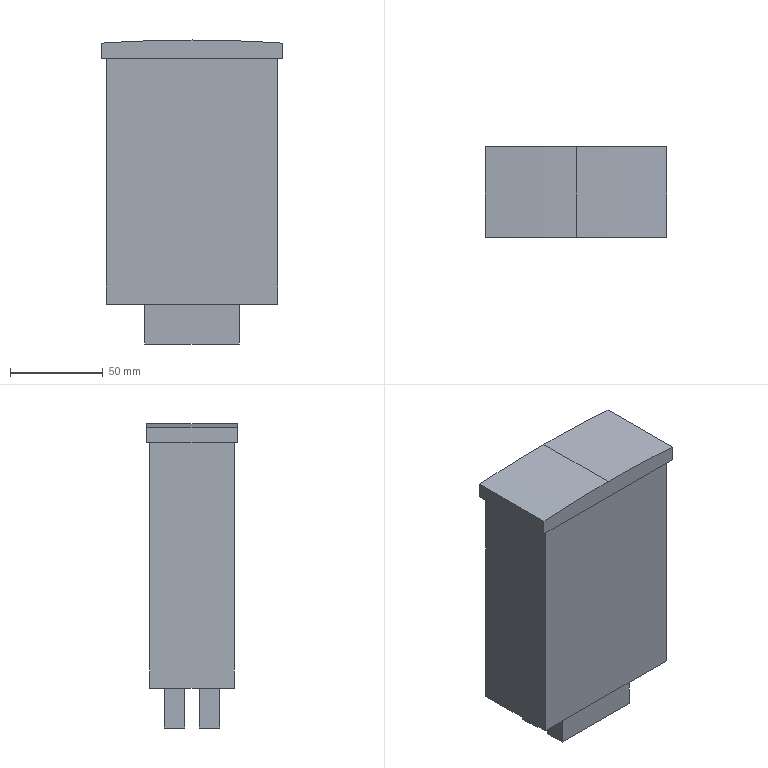Part | SolidWorks | features BaseBody 1 | 1 solid | 22 faces | box 97.6 x 48.9 x 163.5 mm | volume 620484 mm3 | plane 20 | cylinder 2 | commonest cylinder face diameters 1403 x2
STEP:
#1=CARTESIAN_POINT('',(0.,-24.45,71.));
#2=VERTEX_POINT('',#1);
#3=CARTESIAN_POINT('',(-48.8,-24.45,69.3));
#4=VERTEX_POINT('',#3);
#5=CARTESIAN_POINT('',(0.,-24.45,-630.274));
#6=DIRECTION('',(0.,-1.,0.));
#7=DIRECTION('',(0.,0.,1.));
#8=AXIS2_PLACEMENT_3D('',#5,#6,#7);
#9=CIRCLE('',#8,701.274);
#10=EDGE_CURVE('',#2,#4,#9,.T.);
#11=ORIENTED_EDGE('',*,*,#10,.F.);
#12=CARTESIAN_POINT('',(0.,24.45,71.));
#13=VERTEX_POINT('',#12);
#14=CARTESIAN_POINT('',(0.,-24.45,71.));
#15=DIRECTION('',(0.,1.,0.));
#16=VECTOR('',#15,1000.);
#17=LINE('',#14,#16);
#18=EDGE_CURVE('',#2,#13,#17,.T.);
#19=ORIENTED_EDGE('',*,*,#18,.T.);
#20=CARTESIAN_POINT('',(-48.8,24.45,69.3));
#21=VERTEX_POINT('',#20);
#22=CARTESIAN_POINT('',(0.,24.45,-630.274));
#23=DIRECTION('',(0.,-1.,0.));
#24=DIRECTION('',(0.,0.,1.));
#25=AXIS2_PLACEMENT_3D('',#22,#23,#24);
#26=CIRCLE('',#25,701.274);
#27=EDGE_CURVE('',#13,#21,#26,.T.);
#28=ORIENTED_EDGE('',*,*,#27,.T.);
#29=CARTESIAN_POINT('',(-48.8,-24.45,69.3));
#30=DIRECTION('',(0.,1.,0.));
#31=VECTOR('',#30,1000.);
#32=LINE('',#29,#31);
#33=EDGE_CURVE('',#4,#21,#32,.T.);
#34=ORIENTED_EDGE('',*,*,#33,.F.);
#35=EDGE_LOOP('',(#11,#19,#28,#34));
#36=FACE_OUTER_BOUND('',#35,.T.);
#37=CARTESIAN_POINT('',(0.,-24.45,-630.274));
#38=DIRECTION('',(0.,1.,0.));
#39=DIRECTION('',(0.,0.,1.));
#40=AXIS2_PLACEMENT_3D('',#37,#38,#39);
#41=CYLINDRICAL_SURFACE('',#40,701.274);
#42=ADVANCED_FACE('',(#36),#41,.T.);
#43=CARTESIAN_POINT('',(-25.5,-15.,-92.5));
#44=VERTEX_POINT('',#43);
#45=CARTESIAN_POINT('',(-25.5,-4.,-92.5));
#46=VERTEX_POINT('',#45);
#47=CARTESIAN_POINT('',(-25.5,-15.,-92.5));
#48=DIRECTION('',(0.,1.,0.));
#49=VECTOR('',#48,1000.);
#50=LINE('',#47,#49);
#51=EDGE_CURVE('',#44,#46,#50,.T.);
#52=ORIENTED_EDGE('',*,*,#51,.T.);
#53=CARTESIAN_POINT('',(25.5,-4.,-92.5));
#54=VERTEX_POINT('',#53);
#55=CARTESIAN_POINT('',(25.5,-4.,-92.5));
#56=DIRECTION('',(1.,0.,0.));
#57=VECTOR('',#56,1000.);
#58=LINE('',#55,#57);
#59=EDGE_CURVE('',#46,#54,#58,.T.);
#60=ORIENTED_EDGE('',*,*,#59,.T.);
#61=CARTESIAN_POINT('',(25.5,-15.,-92.5));
#62=VERTEX_POINT('',#61);
#63=CARTESIAN_POINT('',(25.5,-15.,-92.5));
#64=DIRECTION('',(0.,-1.,0.));
#65=VECTOR('',#64,1000.);
#66=LINE('',#63,#65);
#67=EDGE_CURVE('',#54,#62,#66,.T.);
#68=ORIENTED_EDGE('',*,*,#67,.T.);
#69=CARTESIAN_POINT('',(25.5,-15.,-92.5));
#70=DIRECTION('',(-1.,0.,0.));
#71=VECTOR('',#70,1000.);
#72=LINE('',#69,#71);
#73=EDGE_CURVE('',#62,#44,#72,.T.);
#74=ORIENTED_EDGE('',*,*,#73,.T.);
#75=EDGE_LOOP('',(#52,#60,#68,#74));
#76=FACE_OUTER_BOUND('',#75,.T.);
#77=CARTESIAN_POINT('',(0.,0.,-92.5));
#78=DIRECTION('',(0.,0.,1.));
#79=DIRECTION('',(1.,0.,0.));
#80=AXIS2_PLACEMENT_3D('',#77,#78,#79);
#81=PLANE('',#80);
#82=ADVANCED_FACE('',(#76),#81,.F.);
#83=CARTESIAN_POINT('',(25.5,-15.,-71.));
#84=VERTEX_POINT('',#83);
#85=CARTESIAN_POINT('',(-25.5,-15.,-71.));
#86=VERTEX_POINT('',#85);
#87=CARTESIAN_POINT('',(25.5,-15.,-71.));
#88=DIRECTION('',(-1.,0.,0.));
#89=VECTOR('',#88,1000.);
#90=LINE('',#87,#89);
#91=EDGE_CURVE('',#84,#86,#90,.T.);
#92=ORIENTED_EDGE('',*,*,#91,.T.);
#93=CARTESIAN_POINT('',(-25.5,-15.,-92.5));
#94=DIRECTION('',(0.,0.,1.));
#95=VECTOR('',#94,1000.);
#96=LINE('',#93,#95);
#97=EDGE_CURVE('',#44,#86,#96,.T.);
#98=ORIENTED_EDGE('',*,*,#97,.F.);
#99=ORIENTED_EDGE('',*,*,#73,.F.);
#100=CARTESIAN_POINT('',(25.5,-15.,-92.5));
#101=DIRECTION('',(0.,0.,1.));
#102=VECTOR('',#101,1000.);
#103=LINE('',#100,#102);
#104=EDGE_CURVE('',#62,#84,#103,.T.);
#105=ORIENTED_EDGE('',*,*,#104,.T.);
#106=EDGE_LOOP('',(#92,#98,#99,#105));
#107=FACE_OUTER_BOUND('',#106,.T.);
#108=CARTESIAN_POINT('',(25.5,-15.,-92.5));
#109=DIRECTION('',(0.,1.,0.));
#110=DIRECTION('',(1.,0.,0.));
#111=AXIS2_PLACEMENT_3D('',#108,#109,#110);
#112=PLANE('',#111);
#113=ADVANCED_FACE('',(#107),#112,.F.);
#114=CARTESIAN_POINT('',(25.5,-4.,-71.));
#115=VERTEX_POINT('',#114);
#116=CARTESIAN_POINT('',(25.5,-15.,-71.));
#117=DIRECTION('',(0.,-1.,0.));
#118=VECTOR('',#117,1000.);
#119=LINE('',#116,#118);
#120=EDGE_CURVE('',#115,#84,#119,.T.);
#121=ORIENTED_EDGE('',*,*,#120,.T.);
#122=ORIENTED_EDGE('',*,*,#104,.F.);
#123=ORIENTED_EDGE('',*,*,#67,.F.);
#124=CARTESIAN_POINT('',(25.5,-4.,-92.5));
#125=DIRECTION('',(0.,0.,1.));
#126=VECTOR('',#125,1000.);
#127=LINE('',#124,#126);
#128=EDGE_CURVE('',#54,#115,#127,.T.);
#129=ORIENTED_EDGE('',*,*,#128,.T.);
#130=EDGE_LOOP('',(#121,#122,#123,#129));
#131=FACE_OUTER_BOUND('',#130,.T.);
#132=CARTESIAN_POINT('',(25.5,-15.,-92.5));
#133=DIRECTION('',(-1.,0.,0.));
#134=DIRECTION('',(0.,0.,1.));
#135=AXIS2_PLACEMENT_3D('',#132,#133,#134);
#136=PLANE('',#135);
#137=ADVANCED_FACE('',(#131),#136,.F.);
#138=CARTESIAN_POINT('',(-25.5,-4.,-71.));
#139=VERTEX_POINT('',#138);
#140=CARTESIAN_POINT('',(25.5,-4.,-71.));
#141=DIRECTION('',(1.,0.,0.));
#142=VECTOR('',#141,1000.);
#143=LINE('',#140,#142);
#144=EDGE_CURVE('',#139,#115,#143,.T.);
#145=ORIENTED_EDGE('',*,*,#144,.T.);
#146=ORIENTED_EDGE('',*,*,#128,.F.);
#147=ORIENTED_EDGE('',*,*,#59,.F.);
#148=CARTESIAN_POINT('',(-25.5,-4.,-92.5));
#149=DIRECTION('',(0.,0.,1.));
#150=VECTOR('',#149,1000.);
#151=LINE('',#148,#150);
#152=EDGE_CURVE('',#46,#139,#151,.T.);
#153=ORIENTED_EDGE('',*,*,#152,.T.);
#154=EDGE_LOOP('',(#145,#146,#147,#153));
#155=FACE_OUTER_BOUND('',#154,.T.);
#156=CARTESIAN_POINT('',(25.5,-4.,-92.5));
#157=DIRECTION('',(0.,-1.,0.));
#158=DIRECTION('',(-1.,0.,0.));
#159=AXIS2_PLACEMENT_3D('',#156,#157,#158);
#160=PLANE('',#159);
#161=ADVANCED_FACE('',(#155),#160,.F.);
#162=CARTESIAN_POINT('',(-25.5,-15.,-71.));
#163=DIRECTION('',(0.,1.,0.));
#164=VECTOR('',#163,1000.);
#165=LINE('',#162,#164);
#166=EDGE_CURVE('',#86,#139,#165,.T.);
#167=ORIENTED_EDGE('',*,*,#166,.T.);
#168=ORIENTED_EDGE('',*,*,#152,.F.);
#169=ORIENTED_EDGE('',*,*,#51,.F.);
#170=ORIENTED_EDGE('',*,*,#97,.T.);
#171=EDGE_LOOP('',(#167,#168,#169,#170));
#172=FACE_OUTER_BOUND('',#171,.T.);
#173=CARTESIAN_POINT('',(-25.5,-15.,-92.5));
#174=DIRECTION('',(1.,0.,0.));
#175=DIRECTION('',(0.,-1.,0.));
#176=AXIS2_PLACEMENT_3D('',#173,#174,#175);
#177=PLANE('',#176);
#178=ADVANCED_FACE('',(#172),#177,.F.);
#179=CARTESIAN_POINT('',(-25.5,4.,-92.5));
#180=VERTEX_POINT('',#179);
#181=CARTESIAN_POINT('',(-25.5,15.,-92.5));
#182=VERTEX_POINT('',#181);
#183=CARTESIAN_POINT('',(-25.5,4.,-92.5));
#184=DIRECTION('',(0.,1.,0.));
#185=VECTOR('',#184,1000.);
#186=LINE('',#183,#185);
#187=EDGE_CURVE('',#180,#182,#186,.T.);
#188=ORIENTED_EDGE('',*,*,#187,.T.);
#189=CARTESIAN_POINT('',(25.5,15.,-92.5));
#190=VERTEX_POINT('',#189);
#191=CARTESIAN_POINT('',(25.5,15.,-92.5));
#192=DIRECTION('',(1.,0.,0.));
#193=VECTOR('',#192,1000.);
#194=LINE('',#191,#193);
#195=EDGE_CURVE('',#182,#190,#194,.T.);
#196=ORIENTED_EDGE('',*,*,#195,.T.);
#197=CARTESIAN_POINT('',(25.5,4.,-92.5));
#198=VERTEX_POINT('',#197);
#199=CARTESIAN_POINT('',(25.5,4.,-92.5));
#200=DIRECTION('',(0.,-1.,0.));
#201=VECTOR('',#200,1000.);
#202=LINE('',#199,#201);
#203=EDGE_CURVE('',#190,#198,#202,.T.);
#204=ORIENTED_EDGE('',*,*,#203,.T.);
#205=CARTESIAN_POINT('',(25.5,4.,-92.5));
#206=DIRECTION('',(-1.,0.,0.));
#207=VECTOR('',#206,1000.);
#208=LINE('',#205,#207);
#209=EDGE_CURVE('',#198,#180,#208,.T.);
#210=ORIENTED_EDGE('',*,*,#209,.T.);
#211=EDGE_LOOP('',(#188,#196,#204,#210));
#212=FACE_OUTER_BOUND('',#211,.T.);
#213=CARTESIAN_POINT('',(0.,0.,-92.5));
#214=DIRECTION('',(0.,0.,1.));
#215=DIRECTION('',(1.,0.,0.));
#216=AXIS2_PLACEMENT_3D('',#213,#214,#215);
#217=PLANE('',#216);
#218=ADVANCED_FACE('',(#212),#217,.F.);
#219=CARTESIAN_POINT('',(25.5,4.,-71.));
#220=VERTEX_POINT('',#219);
#221=CARTESIAN_POINT('',(-25.5,4.,-71.));
#222=VERTEX_POINT('',#221);
#223=CARTESIAN_POINT('',(25.5,4.,-71.));
#224=DIRECTION('',(-1.,0.,0.));
#225=VECTOR('',#224,1000.);
#226=LINE('',#223,#225);
#227=EDGE_CURVE('',#220,#222,#226,.T.);
#228=ORIENTED_EDGE('',*,*,#227,.T.);
#229=CARTESIAN_POINT('',(-25.5,4.,-92.5));
#230=DIRECTION('',(0.,0.,1.));
#231=VECTOR('',#230,1000.);
#232=LINE('',#229,#231);
#233=EDGE_CURVE('',#180,#222,#232,.T.);
#234=ORIENTED_EDGE('',*,*,#233,.F.);
#235=ORIENTED_EDGE('',*,*,#209,.F.);
#236=CARTESIAN_POINT('',(25.5,4.,-92.5));
#237=DIRECTION('',(0.,0.,1.));
#238=VECTOR('',#237,1000.);
#239=LINE('',#236,#238);
#240=EDGE_CURVE('',#198,#220,#239,.T.);
#241=ORIENTED_EDGE('',*,*,#240,.T.);
#242=EDGE_LOOP('',(#228,#234,#235,#241));
#243=FACE_OUTER_BOUND('',#242,.T.);
#244=CARTESIAN_POINT('',(25.5,4.,-92.5));
#245=DIRECTION('',(0.,1.,0.));
#246=DIRECTION('',(1.,0.,0.));
#247=AXIS2_PLACEMENT_3D('',#244,#245,#246);
#248=PLANE('',#247);
#249=ADVANCED_FACE('',(#243),#248,.F.);
#250=CARTESIAN_POINT('',(25.5,15.,-71.));
#251=VERTEX_POINT('',#250);
#252=CARTESIAN_POINT('',(25.5,4.,-71.));
#253=DIRECTION('',(0.,-1.,0.));
#254=VECTOR('',#253,1000.);
#255=LINE('',#252,#254);
#256=EDGE_CURVE('',#251,#220,#255,.T.);
#257=ORIENTED_EDGE('',*,*,#256,.T.);
#258=ORIENTED_EDGE('',*,*,#240,.F.);
#259=ORIENTED_EDGE('',*,*,#203,.F.);
#260=CARTESIAN_POINT('',(25.5,15.,-92.5));
#261=DIRECTION('',(0.,0.,1.));
#262=VECTOR('',#261,1000.);
#263=LINE('',#260,#262);
#264=EDGE_CURVE('',#190,#251,#263,.T.);
#265=ORIENTED_EDGE('',*,*,#264,.T.);
#266=EDGE_LOOP('',(#257,#258,#259,#265));
#267=FACE_OUTER_BOUND('',#266,.T.);
#268=CARTESIAN_POINT('',(25.5,4.,-92.5));
#269=DIRECTION('',(-1.,0.,0.));
#270=DIRECTION('',(0.,0.,1.));
#271=AXIS2_PLACEMENT_3D('',#268,#269,#270);
#272=PLANE('',#271);
#273=ADVANCED_FACE('',(#267),#272,.F.);
#274=CARTESIAN_POINT('',(-25.5,15.,-71.));
#275=VERTEX_POINT('',#274);
#276=CARTESIAN_POINT('',(25.5,15.,-71.));
#277=DIRECTION('',(1.,0.,0.));
#278=VECTOR('',#277,1000.);
#279=LINE('',#276,#278);
#280=EDGE_CURVE('',#275,#251,#279,.T.);
#281=ORIENTED_EDGE('',*,*,#280,.T.);
#282=ORIENTED_EDGE('',*,*,#264,.F.);
#283=ORIENTED_EDGE('',*,*,#195,.F.);
#284=CARTESIAN_POINT('',(-25.5,15.,-92.5));
#285=DIRECTION('',(0.,0.,1.));
#286=VECTOR('',#285,1000.);
#287=LINE('',#284,#286);
#288=EDGE_CURVE('',#182,#275,#287,.T.);
#289=ORIENTED_EDGE('',*,*,#288,.T.);
#290=EDGE_LOOP('',(#281,#282,#283,#289));
#291=FACE_OUTER_BOUND('',#290,.T.);
#292=CARTESIAN_POINT('',(25.5,15.,-92.5));
#293=DIRECTION('',(0.,-1.,0.));
#294=DIRECTION('',(0.,0.,-1.));
#295=AXIS2_PLACEMENT_3D('',#292,#293,#294);
#296=PLANE('',#295);
#297=ADVANCED_FACE('',(#291),#296,.F.);
#298=CARTESIAN_POINT('',(-25.5,4.,-71.));
#299=DIRECTION('',(0.,1.,0.));
#300=VECTOR('',#299,1000.);
#301=LINE('',#298,#300);
#302=EDGE_CURVE('',#222,#275,#301,.T.);
#303=ORIENTED_EDGE('',*,*,#302,.T.);
#304=ORIENTED_EDGE('',*,*,#288,.F.);
#305=ORIENTED_EDGE('',*,*,#187,.F.);
#306=ORIENTED_EDGE('',*,*,#233,.T.);
#307=EDGE_LOOP('',(#303,#304,#305,#306));
#308=FACE_OUTER_BOUND('',#307,.T.);
#309=CARTESIAN_POINT('',(-25.5,4.,-92.5));
#310=DIRECTION('',(1.,0.,0.));
#311=DIRECTION('',(0.,1.,0.));
#312=AXIS2_PLACEMENT_3D('',#309,#310,#311);
#313=PLANE('',#312);
#314=ADVANCED_FACE('',(#308),#313,.F.);
#315=CARTESIAN_POINT('',(48.8,24.45,69.3));
#316=VERTEX_POINT('',#315);
#317=CARTESIAN_POINT('',(0.,24.45,-630.274));
#318=DIRECTION('',(0.,-1.,0.));
#319=DIRECTION('',(0.,0.,1.));
#320=AXIS2_PLACEMENT_3D('',#317,#318,#319);
#321=CIRCLE('',#320,701.274);
#322=EDGE_CURVE('',#316,#13,#321,.T.);
#323=ORIENTED_EDGE('',*,*,#322,.F.);
#324=CARTESIAN_POINT('',(48.8,24.45,61.));
#325=VERTEX_POINT('',#324);
#326=CARTESIAN_POINT('',(48.8,24.45,61.));
#327=DIRECTION('',(0.,0.,1.));
#328=VECTOR('',#327,1000.);
#329=LINE('',#326,#328);
#330=EDGE_CURVE('',#325,#316,#329,.T.);
#331=ORIENTED_EDGE('',*,*,#330,.F.);
#332=CARTESIAN_POINT('',(-48.8,24.45,61.));
#333=VERTEX_POINT('',#332);
#334=CARTESIAN_POINT('',(-48.8,24.45,61.));
#335=DIRECTION('',(-1.,0.,0.));
#336=VECTOR('',#335,1000.);
#337=LINE('',#334,#336);
#338=EDGE_CURVE('',#325,#333,#337,.T.);
#339=ORIENTED_EDGE('',*,*,#338,.T.);
#340=CARTESIAN_POINT('',(-48.8,24.45,61.));
#341=DIRECTION('',(0.,0.,1.));
#342=VECTOR('',#341,1000.);
#343=LINE('',#340,#342);
#344=EDGE_CURVE('',#333,#21,#343,.T.);
#345=ORIENTED_EDGE('',*,*,#344,.T.);
#346=ORIENTED_EDGE('',*,*,#27,.F.);
#347=EDGE_LOOP('',(#323,#331,#339,#345,#346));
#348=FACE_OUTER_BOUND('',#347,.T.);
#349=CARTESIAN_POINT('',(-48.8,24.45,61.));
#350=DIRECTION('',(0.,1.,0.));
#351=DIRECTION('',(1.,0.,0.));
#352=AXIS2_PLACEMENT_3D('',#349,#350,#351);
#353=PLANE('',#352);
#354=ADVANCED_FACE('',(#348),#353,.T.);
#355=ORIENTED_EDGE('',*,*,#33,.T.);
#356=ORIENTED_EDGE('',*,*,#344,.F.);
#357=CARTESIAN_POINT('',(-48.8,-24.45,61.));
#358=VERTEX_POINT('',#357);
#359=CARTESIAN_POINT('',(-48.8,-24.45,61.));
#360=DIRECTION('',(0.,-1.,0.));
#361=VECTOR('',#360,1000.);
#362=LINE('',#359,#361);
#363=EDGE_CURVE('',#333,#358,#362,.T.);
#364=ORIENTED_EDGE('',*,*,#363,.T.);
#365=CARTESIAN_POINT('',(-48.8,-24.45,61.));
#366=DIRECTION('',(0.,0.,1.));
#367=VECTOR('',#366,1000.);
#368=LINE('',#365,#367);
#369=EDGE_CURVE('',#358,#4,#368,.T.);
#370=ORIENTED_EDGE('',*,*,#369,.T.);
#371=EDGE_LOOP('',(#355,#356,#364,#370));
#372=FACE_OUTER_BOUND('',#371,.T.);
#373=CARTESIAN_POINT('',(-48.8,-24.45,61.));
#374=DIRECTION('',(-1.,0.,0.));
#375=DIRECTION('',(0.,0.,1.));
#376=AXIS2_PLACEMENT_3D('',#373,#374,#375);
#377=PLANE('',#376);
#378=ADVANCED_FACE('',(#372),#377,.T.);
#379=CARTESIAN_POINT('',(48.8,-24.45,61.));
#380=VERTEX_POINT('',#379);
#381=CARTESIAN_POINT('',(48.8,-24.45,69.3));
#382=VERTEX_POINT('',#381);
#383=CARTESIAN_POINT('',(48.8,-24.45,61.));
#384=DIRECTION('',(0.,0.,1.));
#385=VECTOR('',#384,1000.);
#386=LINE('',#383,#385);
#387=EDGE_CURVE('',#380,#382,#386,.T.);
#388=ORIENTED_EDGE('',*,*,#387,.T.);
#389=CARTESIAN_POINT('',(0.,-24.45,-630.274));
#390=DIRECTION('',(0.,-1.,0.));
#391=DIRECTION('',(0.,0.,1.));
#392=AXIS2_PLACEMENT_3D('',#389,#390,#391);
#393=CIRCLE('',#392,701.274);
#394=EDGE_CURVE('',#382,#2,#393,.T.);
#395=ORIENTED_EDGE('',*,*,#394,.T.);
#396=ORIENTED_EDGE('',*,*,#10,.T.);
#397=ORIENTED_EDGE('',*,*,#369,.F.);
#398=CARTESIAN_POINT('',(-48.8,-24.45,61.));
#399=DIRECTION('',(1.,0.,0.));
#400=VECTOR('',#399,1000.);
#401=LINE('',#398,#400);
#402=EDGE_CURVE('',#358,#380,#401,.T.);
#403=ORIENTED_EDGE('',*,*,#402,.T.);
#404=EDGE_LOOP('',(#388,#395,#396,#397,#403));
#405=FACE_OUTER_BOUND('',#404,.T.);
#406=CARTESIAN_POINT('',(-48.8,-24.45,61.));
#407=DIRECTION('',(0.,-1.,0.));
#408=DIRECTION('',(0.,0.,-1.));
#409=AXIS2_PLACEMENT_3D('',#406,#407,#408);
#410=PLANE('',#409);
#411=ADVANCED_FACE('',(#405),#410,.T.);
#412=CARTESIAN_POINT('',(48.8,-24.45,69.3));
#413=DIRECTION('',(0.,1.,0.));
#414=VECTOR('',#413,1000.);
#415=LINE('',#412,#414);
#416=EDGE_CURVE('',#382,#316,#415,.T.);
#417=ORIENTED_EDGE('',*,*,#416,.F.);
#418=ORIENTED_EDGE('',*,*,#387,.F.);
#419=CARTESIAN_POINT('',(48.8,-24.45,61.));
#420=DIRECTION('',(0.,1.,0.));
#421=VECTOR('',#420,1000.);
#422=LINE('',#419,#421);
#423=EDGE_CURVE('',#380,#325,#422,.T.);
#424=ORIENTED_EDGE('',*,*,#423,.T.);
#425=ORIENTED_EDGE('',*,*,#330,.T.);
#426=EDGE_LOOP('',(#417,#418,#424,#425));
#427=FACE_OUTER_BOUND('',#426,.T.);
#428=CARTESIAN_POINT('',(48.8,-24.45,61.));
#429=DIRECTION('',(1.,0.,0.));
#430=DIRECTION('',(0.,1.,0.));
#431=AXIS2_PLACEMENT_3D('',#428,#429,#430);
#432=PLANE('',#431);
#433=ADVANCED_FACE('',(#427),#432,.T.);
#434=CARTESIAN_POINT('',(46.,22.7,61.));
#435=VERTEX_POINT('',#434);
#436=CARTESIAN_POINT('',(46.,-22.7,61.));
#437=VERTEX_POINT('',#436);
#438=CARTESIAN_POINT('',(46.,-22.7,61.));
#439=DIRECTION('',(0.,-1.,0.));
#440=VECTOR('',#439,1000.);
#441=LINE('',#438,#440);
#442=EDGE_CURVE('',#435,#437,#441,.T.);
#443=ORIENTED_EDGE('',*,*,#442,.F.);
#444=CARTESIAN_POINT('',(-46.,22.7,61.));
#445=VERTEX_POINT('',#444);
#446=CARTESIAN_POINT('',(-46.,22.7,61.));
#447=DIRECTION('',(1.,0.,0.));
#448=VECTOR('',#447,1000.);
#449=LINE('',#446,#448);
#450=EDGE_CURVE('',#445,#435,#449,.T.);
#451=ORIENTED_EDGE('',*,*,#450,.F.);
#452=CARTESIAN_POINT('',(-46.,-22.7,61.));
#453=VERTEX_POINT('',#452);
#454=CARTESIAN_POINT('',(-46.,-22.7,61.));
#455=DIRECTION('',(0.,1.,0.));
#456=VECTOR('',#455,1000.);
#457=LINE('',#454,#456);
#458=EDGE_CURVE('',#453,#445,#457,.T.);
#459=ORIENTED_EDGE('',*,*,#458,.F.);
#460=CARTESIAN_POINT('',(-46.,-22.7,61.));
#461=DIRECTION('',(-1.,0.,0.));
#462=VECTOR('',#461,1000.);
#463=LINE('',#460,#462);
#464=EDGE_CURVE('',#437,#453,#463,.T.);
#465=ORIENTED_EDGE('',*,*,#464,.F.);
#466=EDGE_LOOP('',(#443,#451,#459,#465));
#467=FACE_BOUND('',#466,.T.);
#468=ORIENTED_EDGE('',*,*,#423,.F.);
#469=ORIENTED_EDGE('',*,*,#402,.F.);
#470=ORIENTED_EDGE('',*,*,#363,.F.);
#471=ORIENTED_EDGE('',*,*,#338,.F.);
#472=EDGE_LOOP('',(#468,#469,#470,#471));
#473=FACE_OUTER_BOUND('',#472,.T.);
#474=CARTESIAN_POINT('',(0.,0.,61.));
#475=DIRECTION('',(0.,0.,-1.));
#476=DIRECTION('',(0.,-1.,0.));
#477=AXIS2_PLACEMENT_3D('',#474,#475,#476);
#478=PLANE('',#477);
#479=ADVANCED_FACE('',(#467,#473),#478,.T.);
#480=CARTESIAN_POINT('',(46.,-22.7,-71.));
#481=VERTEX_POINT('',#480);
#482=CARTESIAN_POINT('',(46.,-22.7,71.));
#483=DIRECTION('',(0.,0.,-1.));
#484=VECTOR('',#483,1000.);
#485=LINE('',#482,#484);
#486=EDGE_CURVE('',#437,#481,#485,.T.);
#487=ORIENTED_EDGE('',*,*,#486,.F.);
#488=ORIENTED_EDGE('',*,*,#464,.T.);
#489=CARTESIAN_POINT('',(-46.,-22.7,-71.));
#490=VERTEX_POINT('',#489);
#491=CARTESIAN_POINT('',(-46.,-22.7,71.));
#492=DIRECTION('',(0.,0.,-1.));
#493=VECTOR('',#492,1000.);
#494=LINE('',#491,#493);
#495=EDGE_CURVE('',#453,#490,#494,.T.);
#496=ORIENTED_EDGE('',*,*,#495,.T.);
#497=CARTESIAN_POINT('',(-46.,-22.7,-71.));
#498=DIRECTION('',(1.,0.,0.));
#499=VECTOR('',#498,1000.);
#500=LINE('',#497,#499);
#501=EDGE_CURVE('',#490,#481,#500,.T.);
#502=ORIENTED_EDGE('',*,*,#501,.T.);
#503=EDGE_LOOP('',(#487,#488,#496,#502));
#504=FACE_OUTER_BOUND('',#503,.T.);
#505=CARTESIAN_POINT('',(-46.,-22.7,71.));
#506=DIRECTION('',(0.,1.,0.));
#507=DIRECTION('',(1.,0.,0.));
#508=AXIS2_PLACEMENT_3D('',#505,#506,#507);
#509=PLANE('',#508);
#510=ADVANCED_FACE('',(#504),#509,.F.);
#511=ORIENTED_EDGE('',*,*,#495,.F.);
#512=ORIENTED_EDGE('',*,*,#458,.T.);
#513=CARTESIAN_POINT('',(-46.,22.7,-71.));
#514=VERTEX_POINT('',#513);
#515=CARTESIAN_POINT('',(-46.,22.7,71.));
#516=DIRECTION('',(0.,0.,-1.));
#517=VECTOR('',#516,1000.);
#518=LINE('',#515,#517);
#519=EDGE_CURVE('',#445,#514,#518,.T.);
#520=ORIENTED_EDGE('',*,*,#519,.T.);
#521=CARTESIAN_POINT('',(-46.,-22.7,-71.));
#522=DIRECTION('',(0.,-1.,0.));
#523=VECTOR('',#522,1000.);
#524=LINE('',#521,#523);
#525=EDGE_CURVE('',#514,#490,#524,.T.);
#526=ORIENTED_EDGE('',*,*,#525,.T.);
#527=EDGE_LOOP('',(#511,#512,#520,#526));
#528=FACE_OUTER_BOUND('',#527,.T.);
#529=CARTESIAN_POINT('',(-46.,-22.7,71.));
#530=DIRECTION('',(1.,0.,0.));
#531=DIRECTION('',(0.,1.,0.));
#532=AXIS2_PLACEMENT_3D('',#529,#530,#531);
#533=PLANE('',#532);
#534=ADVANCED_FACE('',(#528),#533,.F.);
#535=ORIENTED_EDGE('',*,*,#519,.F.);
#536=ORIENTED_EDGE('',*,*,#450,.T.);
#537=CARTESIAN_POINT('',(46.,22.7,-71.));
#538=VERTEX_POINT('',#537);
#539=CARTESIAN_POINT('',(46.,22.7,71.));
#540=DIRECTION('',(0.,0.,-1.));
#541=VECTOR('',#540,1000.);
#542=LINE('',#539,#541);
#543=EDGE_CURVE('',#435,#538,#542,.T.);
#544=ORIENTED_EDGE('',*,*,#543,.T.);
#545=CARTESIAN_POINT('',(-46.,22.7,-71.));
#546=DIRECTION('',(-1.,0.,0.));
#547=VECTOR('',#546,1000.);
#548=LINE('',#545,#547);
#549=EDGE_CURVE('',#538,#514,#548,.T.);
#550=ORIENTED_EDGE('',*,*,#549,.T.);
#551=EDGE_LOOP('',(#535,#536,#544,#550));
#552=FACE_OUTER_BOUND('',#551,.T.);
#553=CARTESIAN_POINT('',(-46.,22.7,71.));
#554=DIRECTION('',(0.,-1.,0.));
#555=DIRECTION('',(0.,0.,-1.));
#556=AXIS2_PLACEMENT_3D('',#553,#554,#555);
#557=PLANE('',#556);
#558=ADVANCED_FACE('',(#552),#557,.F.);
#559=ORIENTED_EDGE('',*,*,#543,.F.);
#560=ORIENTED_EDGE('',*,*,#442,.T.);
#561=ORIENTED_EDGE('',*,*,#486,.T.);
#562=CARTESIAN_POINT('',(46.,-22.7,-71.));
#563=DIRECTION('',(0.,1.,0.));
#564=VECTOR('',#563,1000.);
#565=LINE('',#562,#564);
#566=EDGE_CURVE('',#481,#538,#565,.T.);
#567=ORIENTED_EDGE('',*,*,#566,.T.);
#568=EDGE_LOOP('',(#559,#560,#561,#567));
#569=FACE_OUTER_BOUND('',#568,.T.);
#570=CARTESIAN_POINT('',(46.,-22.7,71.));
#571=DIRECTION('',(-1.,0.,0.));
#572=DIRECTION('',(0.,0.,1.));
#573=AXIS2_PLACEMENT_3D('',#570,#571,#572);
#574=PLANE('',#573);
#575=ADVANCED_FACE('',(#569),#574,.F.);
#576=ORIENTED_EDGE('',*,*,#144,.F.);
#577=ORIENTED_EDGE('',*,*,#166,.F.);
#578=ORIENTED_EDGE('',*,*,#91,.F.);
#579=ORIENTED_EDGE('',*,*,#120,.F.);
#580=EDGE_LOOP('',(#576,#577,#578,#579));
#581=FACE_BOUND('',#580,.T.);
#582=ORIENTED_EDGE('',*,*,#280,.F.);
#583=ORIENTED_EDGE('',*,*,#302,.F.);
#584=ORIENTED_EDGE('',*,*,#227,.F.);
#585=ORIENTED_EDGE('',*,*,#256,.F.);
#586=EDGE_LOOP('',(#582,#583,#584,#585));
#587=FACE_BOUND('',#586,.T.);
#588=ORIENTED_EDGE('',*,*,#566,.F.);
#589=ORIENTED_EDGE('',*,*,#501,.F.);
#590=ORIENTED_EDGE('',*,*,#525,.F.);
#591=ORIENTED_EDGE('',*,*,#549,.F.);
#592=EDGE_LOOP('',(#588,#589,#590,#591));
#593=FACE_OUTER_BOUND('',#592,.T.);
#594=CARTESIAN_POINT('',(0.,0.,-71.));
#595=DIRECTION('',(0.,0.,-1.));
#596=DIRECTION('',(0.,-1.,0.));
#597=AXIS2_PLACEMENT_3D('',#594,#595,#596);
#598=PLANE('',#597);
#599=ADVANCED_FACE('',(#581,#587,#593),#598,.T.);
#600=ORIENTED_EDGE('',*,*,#18,.F.);
#601=ORIENTED_EDGE('',*,*,#394,.F.);
#602=ORIENTED_EDGE('',*,*,#416,.T.);
#603=ORIENTED_EDGE('',*,*,#322,.T.);
#604=EDGE_LOOP('',(#600,#601,#602,#603));
#605=FACE_OUTER_BOUND('',#604,.T.);
#606=CARTESIAN_POINT('',(0.,-24.45,-630.274));
#607=DIRECTION('',(0.,1.,0.));
#608=DIRECTION('',(0.,0.,1.));
#609=AXIS2_PLACEMENT_3D('',#606,#607,#608);
#610=CYLINDRICAL_SURFACE('',#609,701.274);
#611=ADVANCED_FACE('',(#605),#610,.T.);
#612=CLOSED_SHELL('',(#42,#82,#113,#137,#161,#178,#218,#249,#273,#297,#314,#354,#378,#411,#433,#479,#510,#534,#558,#575,#599,#611));
#613=MANIFOLD_SOLID_BREP('',#612);
#614=CARTESIAN_POINT('',(0.,0.,0.));
#615=DIRECTION('',(0.,0.,1.));
#616=DIRECTION('',(1.,0.,0.));
#617=AXIS2_PLACEMENT_3D('',#614,#615,#616);
#618=(LENGTH_UNIT()NAMED_UNIT(*)SI_UNIT(.MILLI.,.METRE.));
#619=UNCERTAINTY_MEASURE_WITH_UNIT(LENGTH_MEASURE(0.00001),#618,'','');
#620=(NAMED_UNIT(*)PLANE_ANGLE_UNIT()SI_UNIT($,.RADIAN.));
#621=(NAMED_UNIT(*)SI_UNIT($,.STERADIAN.)SOLID_ANGLE_UNIT());
#622=(GEOMETRIC_REPRESENTATION_CONTEXT(3)GLOBAL_UNCERTAINTY_ASSIGNED_CONTEXT((#619))GLOBAL_UNIT_ASSIGNED_CONTEXT((#618,#620,#621))REPRESENTATION_CONTEXT('',''));
#623=ADVANCED_BREP_SHAPE_REPRESENTATION('',(#613,#617),#622);